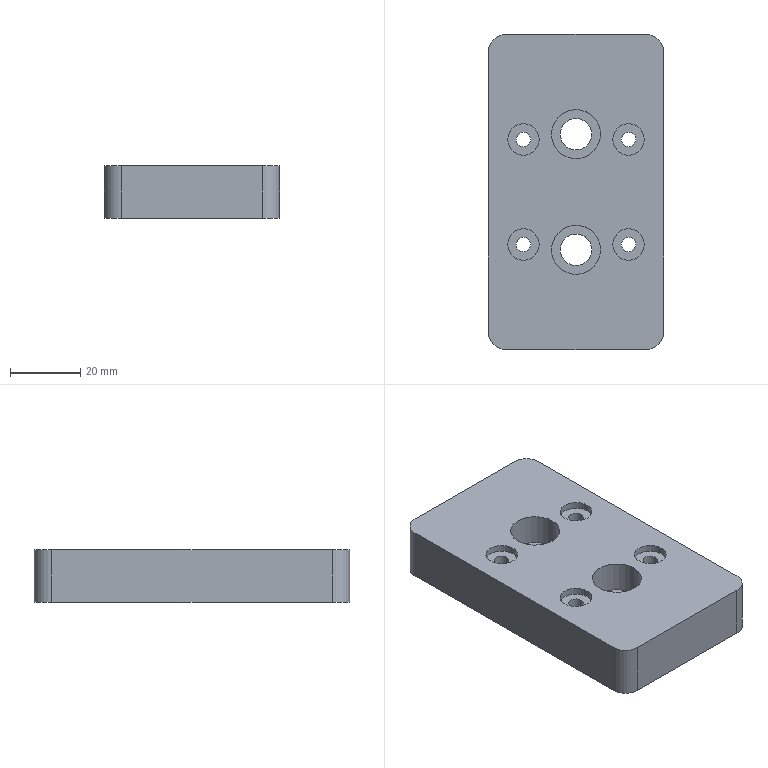Part | STEP file | SN10_012_002_ADAPTADOR | 1 solid | 32 faces | box 50 x 90 x 15 mm | volume 62180 mm3 | cylinder 18 | plane 14 | commonest cylinder face diameters 9 x6 4.134 x4 10 x4 12 x2 14 x2